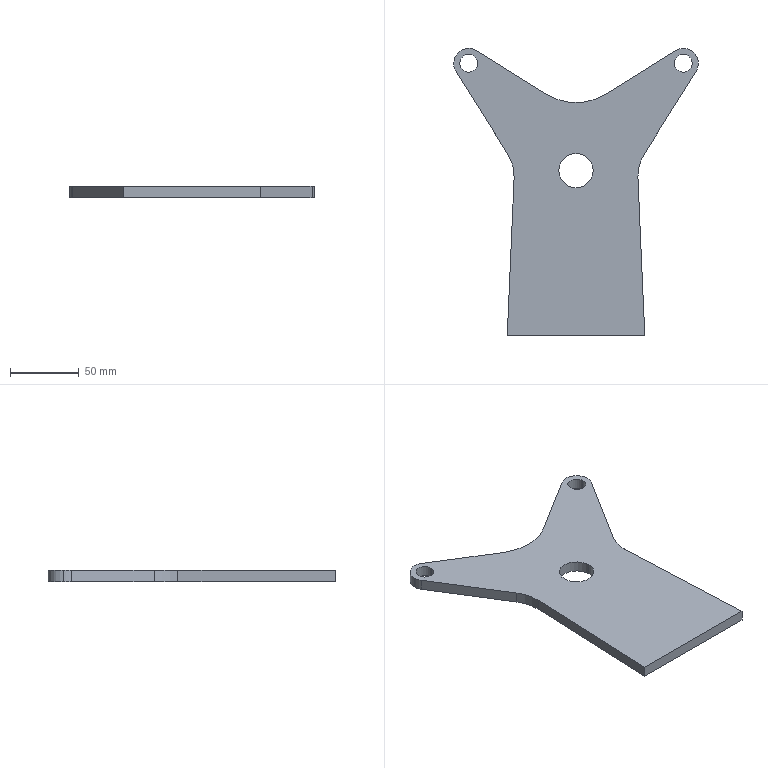Part | SolidWorks | features Extrusion 1 | 1 solid | 22 faces | box 177.818 x 208.909 x 8 mm | volume 156021 mm3 | cylinder 13 | plane 9 | commonest cylinder face diameters 13 x4 21.818 x3 60 x3 25 x2 80 x1
STEP:
#1=CARTESIAN_POINT('',(-84.5,198.,4.));
#2=VERTEX_POINT('',#1);
#3=CARTESIAN_POINT('',(-71.5,198.,4.));
#4=VERTEX_POINT('',#3);
#5=CARTESIAN_POINT('',(-78.,198.,4.));
#6=DIRECTION('',(0.,0.,1.));
#7=DIRECTION('',(-1.,0.,0.));
#8=AXIS2_PLACEMENT_3D('',#5,#6,#7);
#9=CIRCLE('',#8,6.5);
#10=EDGE_CURVE('',#2,#4,#9,.T.);
#11=ORIENTED_EDGE('',*,*,#10,.T.);
#12=CARTESIAN_POINT('',(-71.5,198.,-4.));
#13=VERTEX_POINT('',#12);
#14=CARTESIAN_POINT('',(-71.5,198.,4.));
#15=DIRECTION('',(0.,0.,-1.));
#16=VECTOR('',#15,1000.);
#17=LINE('',#14,#16);
#18=EDGE_CURVE('',#4,#13,#17,.T.);
#19=ORIENTED_EDGE('',*,*,#18,.T.);
#20=CARTESIAN_POINT('',(-84.5,198.,-4.));
#21=VERTEX_POINT('',#20);
#22=CARTESIAN_POINT('',(-78.,198.,-4.));
#23=DIRECTION('',(0.,0.,1.));
#24=DIRECTION('',(-1.,0.,0.));
#25=AXIS2_PLACEMENT_3D('',#22,#23,#24);
#26=CIRCLE('',#25,6.5);
#27=EDGE_CURVE('',#21,#13,#26,.T.);
#28=ORIENTED_EDGE('',*,*,#27,.F.);
#29=CARTESIAN_POINT('',(-84.5,198.,4.));
#30=DIRECTION('',(0.,0.,-1.));
#31=VECTOR('',#30,1000.);
#32=LINE('',#29,#31);
#33=EDGE_CURVE('',#2,#21,#32,.T.);
#34=ORIENTED_EDGE('',*,*,#33,.F.);
#35=EDGE_LOOP('',(#11,#19,#28,#34));
#36=FACE_OUTER_BOUND('',#35,.T.);
#37=CARTESIAN_POINT('',(-78.,198.,4.));
#38=DIRECTION('',(0.,0.,-1.));
#39=DIRECTION('',(-1.,0.,0.));
#40=AXIS2_PLACEMENT_3D('',#37,#38,#39);
#41=CYLINDRICAL_SURFACE('',#40,6.5);
#42=ADVANCED_FACE('',(#36),#41,.F.);
#43=CARTESIAN_POINT('',(-12.5,120.,4.));
#44=VERTEX_POINT('',#43);
#45=CARTESIAN_POINT('',(12.5,120.,4.));
#46=VERTEX_POINT('',#45);
#47=CARTESIAN_POINT('',(0.,120.,4.));
#48=DIRECTION('',(0.,0.,1.));
#49=DIRECTION('',(1.,0.,0.));
#50=AXIS2_PLACEMENT_3D('',#47,#48,#49);
#51=CIRCLE('',#50,12.5);
#52=EDGE_CURVE('',#44,#46,#51,.T.);
#53=ORIENTED_EDGE('',*,*,#52,.T.);
#54=CARTESIAN_POINT('',(12.5,120.,-4.));
#55=VERTEX_POINT('',#54);
#56=CARTESIAN_POINT('',(12.5,120.,4.));
#57=DIRECTION('',(0.,0.,-1.));
#58=VECTOR('',#57,1000.);
#59=LINE('',#56,#58);
#60=EDGE_CURVE('',#46,#55,#59,.T.);
#61=ORIENTED_EDGE('',*,*,#60,.T.);
#62=CARTESIAN_POINT('',(-12.5,120.,-4.));
#63=VERTEX_POINT('',#62);
#64=CARTESIAN_POINT('',(0.,120.,-4.));
#65=DIRECTION('',(0.,0.,1.));
#66=DIRECTION('',(1.,0.,0.));
#67=AXIS2_PLACEMENT_3D('',#64,#65,#66);
#68=CIRCLE('',#67,12.5);
#69=EDGE_CURVE('',#63,#55,#68,.T.);
#70=ORIENTED_EDGE('',*,*,#69,.F.);
#71=CARTESIAN_POINT('',(-12.5,120.,4.));
#72=DIRECTION('',(0.,0.,-1.));
#73=VECTOR('',#72,1000.);
#74=LINE('',#71,#73);
#75=EDGE_CURVE('',#44,#63,#74,.T.);
#76=ORIENTED_EDGE('',*,*,#75,.F.);
#77=EDGE_LOOP('',(#53,#61,#70,#76));
#78=FACE_OUTER_BOUND('',#77,.T.);
#79=CARTESIAN_POINT('',(0.,120.,4.));
#80=DIRECTION('',(0.,0.,-1.));
#81=DIRECTION('',(-1.,0.,0.));
#82=AXIS2_PLACEMENT_3D('',#79,#80,#81);
#83=CYLINDRICAL_SURFACE('',#82,12.5);
#84=ADVANCED_FACE('',(#78),#83,.F.);
#85=CARTESIAN_POINT('',(71.5,198.,4.));
#86=VERTEX_POINT('',#85);
#87=CARTESIAN_POINT('',(84.5,198.,4.));
#88=VERTEX_POINT('',#87);
#89=CARTESIAN_POINT('',(78.,198.,4.));
#90=DIRECTION('',(0.,0.,1.));
#91=DIRECTION('',(1.,0.,0.));
#92=AXIS2_PLACEMENT_3D('',#89,#90,#91);
#93=CIRCLE('',#92,6.5);
#94=EDGE_CURVE('',#86,#88,#93,.T.);
#95=ORIENTED_EDGE('',*,*,#94,.T.);
#96=CARTESIAN_POINT('',(84.5,198.,-4.));
#97=VERTEX_POINT('',#96);
#98=CARTESIAN_POINT('',(84.5,198.,4.));
#99=DIRECTION('',(0.,0.,-1.));
#100=VECTOR('',#99,1000.);
#101=LINE('',#98,#100);
#102=EDGE_CURVE('',#88,#97,#101,.T.);
#103=ORIENTED_EDGE('',*,*,#102,.T.);
#104=CARTESIAN_POINT('',(71.5,198.,-4.));
#105=VERTEX_POINT('',#104);
#106=CARTESIAN_POINT('',(78.,198.,-4.));
#107=DIRECTION('',(0.,0.,1.));
#108=DIRECTION('',(1.,0.,0.));
#109=AXIS2_PLACEMENT_3D('',#106,#107,#108);
#110=CIRCLE('',#109,6.5);
#111=EDGE_CURVE('',#105,#97,#110,.T.);
#112=ORIENTED_EDGE('',*,*,#111,.F.);
#113=CARTESIAN_POINT('',(71.5,198.,4.));
#114=DIRECTION('',(0.,0.,-1.));
#115=VECTOR('',#114,1000.);
#116=LINE('',#113,#115);
#117=EDGE_CURVE('',#86,#105,#116,.T.);
#118=ORIENTED_EDGE('',*,*,#117,.F.);
#119=EDGE_LOOP('',(#95,#103,#112,#118));
#120=FACE_OUTER_BOUND('',#119,.T.);
#121=CARTESIAN_POINT('',(78.,198.,4.));
#122=DIRECTION('',(0.,0.,-1.));
#123=DIRECTION('',(-1.,0.,0.));
#124=AXIS2_PLACEMENT_3D('',#121,#122,#123);
#125=CYLINDRICAL_SURFACE('',#124,6.5);
#126=ADVANCED_FACE('',(#120),#125,.F.);
#127=CARTESIAN_POINT('',(-88.909,198.,4.));
#128=VERTEX_POINT('',#127);
#129=CARTESIAN_POINT('',(-87.252,192.219,4.));
#130=VERTEX_POINT('',#129);
#131=CARTESIAN_POINT('',(-78.,198.,4.));
#132=DIRECTION('',(0.,0.,1.));
#133=DIRECTION('',(-1.,0.,0.));
#134=AXIS2_PLACEMENT_3D('',#131,#132,#133);
#135=CIRCLE('',#134,10.909);
#136=EDGE_CURVE('',#128,#130,#135,.T.);
#137=ORIENTED_EDGE('',*,*,#136,.F.);
#138=CARTESIAN_POINT('',(-88.909,198.,-4.));
#139=VERTEX_POINT('',#138);
#140=CARTESIAN_POINT('',(-88.909,198.,4.));
#141=DIRECTION('',(0.,0.,-1.));
#142=VECTOR('',#141,1000.);
#143=LINE('',#140,#142);
#144=EDGE_CURVE('',#128,#139,#143,.T.);
#145=ORIENTED_EDGE('',*,*,#144,.T.);
#146=CARTESIAN_POINT('',(-87.252,192.219,-4.));
#147=VERTEX_POINT('',#146);
#148=CARTESIAN_POINT('',(-78.,198.,-4.));
#149=DIRECTION('',(0.,0.,1.));
#150=DIRECTION('',(-1.,0.,0.));
#151=AXIS2_PLACEMENT_3D('',#148,#149,#150);
#152=CIRCLE('',#151,10.909);
#153=EDGE_CURVE('',#139,#147,#152,.T.);
#154=ORIENTED_EDGE('',*,*,#153,.T.);
#155=CARTESIAN_POINT('',(-87.252,192.219,4.));
#156=DIRECTION('',(0.,0.,-1.));
#157=VECTOR('',#156,1000.);
#158=LINE('',#155,#157);
#159=EDGE_CURVE('',#130,#147,#158,.T.);
#160=ORIENTED_EDGE('',*,*,#159,.F.);
#161=EDGE_LOOP('',(#137,#145,#154,#160));
#162=FACE_OUTER_BOUND('',#161,.T.);
#163=CARTESIAN_POINT('',(-78.,198.,4.));
#164=DIRECTION('',(0.,0.,-1.));
#165=DIRECTION('',(-1.,0.,0.));
#166=AXIS2_PLACEMENT_3D('',#163,#164,#165);
#167=CYLINDRICAL_SURFACE('',#166,10.909);
#168=ADVANCED_FACE('',(#162),#167,.T.);
#169=CARTESIAN_POINT('',(45.,116.,4.));
#170=VERTEX_POINT('',#169);
#171=CARTESIAN_POINT('',(49.559,131.898,4.));
#172=VERTEX_POINT('',#171);
#173=CARTESIAN_POINT('',(75.,116.,4.));
#174=DIRECTION('',(0.,0.,-1.));
#175=DIRECTION('',(-1.,0.,0.));
#176=AXIS2_PLACEMENT_3D('',#173,#174,#175);
#177=CIRCLE('',#176,30.);
#178=EDGE_CURVE('',#170,#172,#177,.T.);
#179=ORIENTED_EDGE('',*,*,#178,.F.);
#180=CARTESIAN_POINT('',(45.,116.,-4.));
#181=VERTEX_POINT('',#180);
#182=CARTESIAN_POINT('',(45.,116.,4.));
#183=DIRECTION('',(0.,0.,-1.));
#184=VECTOR('',#183,1000.);
#185=LINE('',#182,#184);
#186=EDGE_CURVE('',#170,#181,#185,.T.);
#187=ORIENTED_EDGE('',*,*,#186,.T.);
#188=CARTESIAN_POINT('',(49.559,131.898,-4.));
#189=VERTEX_POINT('',#188);
#190=CARTESIAN_POINT('',(75.,116.,-4.));
#191=DIRECTION('',(0.,0.,-1.));
#192=DIRECTION('',(-1.,0.,0.));
#193=AXIS2_PLACEMENT_3D('',#190,#191,#192);
#194=CIRCLE('',#193,30.);
#195=EDGE_CURVE('',#181,#189,#194,.T.);
#196=ORIENTED_EDGE('',*,*,#195,.T.);
#197=CARTESIAN_POINT('',(49.559,131.898,4.));
#198=DIRECTION('',(0.,0.,-1.));
#199=VECTOR('',#198,1000.);
#200=LINE('',#197,#199);
#201=EDGE_CURVE('',#172,#189,#200,.T.);
#202=ORIENTED_EDGE('',*,*,#201,.F.);
#203=EDGE_LOOP('',(#179,#187,#196,#202));
#204=FACE_OUTER_BOUND('',#203,.T.);
#205=CARTESIAN_POINT('',(75.,116.,4.));
#206=DIRECTION('',(0.,0.,-1.));
#207=DIRECTION('',(-1.,0.,0.));
#208=AXIS2_PLACEMENT_3D('',#205,#206,#207);
#209=CYLINDRICAL_SURFACE('',#208,30.);
#210=ADVANCED_FACE('',(#204),#209,.F.);
#211=ORIENTED_EDGE('',*,*,#52,.F.);
#212=CARTESIAN_POINT('',(0.,120.,4.));
#213=DIRECTION('',(0.,0.,1.));
#214=DIRECTION('',(1.,0.,0.));
#215=AXIS2_PLACEMENT_3D('',#212,#213,#214);
#216=CIRCLE('',#215,12.5);
#217=EDGE_CURVE('',#46,#44,#216,.T.);
#218=ORIENTED_EDGE('',*,*,#217,.F.);
#219=EDGE_LOOP('',(#211,#218));
#220=FACE_BOUND('',#219,.T.);
#221=CARTESIAN_POINT('',(-45.028,114.701,4.));
#222=VERTEX_POINT('',#221);
#223=CARTESIAN_POINT('',(-50.,0.,4.));
#224=VERTEX_POINT('',#223);
#225=CARTESIAN_POINT('',(-50.,0.,4.));
#226=DIRECTION('',(-0.04331,-0.9991,0.));
#227=VECTOR('',#226,1000.);
#228=LINE('',#225,#227);
#229=EDGE_CURVE('',#222,#224,#228,.T.);
#230=ORIENTED_EDGE('',*,*,#229,.T.);
#231=CARTESIAN_POINT('',(50.,0.,4.));
#232=VERTEX_POINT('',#231);
#233=CARTESIAN_POINT('',(50.,0.,4.));
#234=DIRECTION('',(1.,0.,0.));
#235=VECTOR('',#234,1000.);
#236=LINE('',#233,#235);
#237=EDGE_CURVE('',#224,#232,#236,.T.);
#238=ORIENTED_EDGE('',*,*,#237,.T.);
#239=CARTESIAN_POINT('',(45.028,114.701,4.));
#240=VERTEX_POINT('',#239);
#241=CARTESIAN_POINT('',(50.,0.,4.));
#242=DIRECTION('',(-0.04331,0.9991,0.));
#243=VECTOR('',#242,1000.);
#244=LINE('',#241,#243);
#245=EDGE_CURVE('',#232,#240,#244,.T.);
#246=ORIENTED_EDGE('',*,*,#245,.T.);
#247=CARTESIAN_POINT('',(75.,116.,4.));
#248=DIRECTION('',(0.,0.,-1.));
#249=DIRECTION('',(-1.,0.,0.));
#250=AXIS2_PLACEMENT_3D('',#247,#248,#249);
#251=CIRCLE('',#250,30.);
#252=EDGE_CURVE('',#240,#170,#251,.T.);
#253=ORIENTED_EDGE('',*,*,#252,.T.);
#254=ORIENTED_EDGE('',*,*,#178,.T.);
#255=CARTESIAN_POINT('',(87.252,192.219,4.));
#256=VERTEX_POINT('',#255);
#257=CARTESIAN_POINT('',(49.559,131.898,4.));
#258=DIRECTION('',(0.5299,0.848,0.));
#259=VECTOR('',#258,1000.);
#260=LINE('',#257,#259);
#261=EDGE_CURVE('',#172,#256,#260,.T.);
#262=ORIENTED_EDGE('',*,*,#261,.T.);
#263=CARTESIAN_POINT('',(72.219,207.252,4.));
#264=VERTEX_POINT('',#263);
#265=CARTESIAN_POINT('',(78.,198.,4.));
#266=DIRECTION('',(0.,0.,1.));
#267=DIRECTION('',(1.,0.,0.));
#268=AXIS2_PLACEMENT_3D('',#265,#266,#267);
#269=CIRCLE('',#268,10.909);
#270=EDGE_CURVE('',#256,#264,#269,.T.);
#271=ORIENTED_EDGE('',*,*,#270,.T.);
#272=CARTESIAN_POINT('',(21.197,175.369,4.));
#273=VERTEX_POINT('',#272);
#274=CARTESIAN_POINT('',(72.219,207.252,4.));
#275=DIRECTION('',(-0.848,-0.5299,0.));
#276=VECTOR('',#275,1000.);
#277=LINE('',#274,#276);
#278=EDGE_CURVE('',#264,#273,#277,.T.);
#279=ORIENTED_EDGE('',*,*,#278,.T.);
#280=CARTESIAN_POINT('',(-21.197,175.369,4.));
#281=VERTEX_POINT('',#280);
#282=CARTESIAN_POINT('',(0.,209.291,4.));
#283=DIRECTION('',(0.,0.,-1.));
#284=DIRECTION('',(-1.,0.,0.));
#285=AXIS2_PLACEMENT_3D('',#282,#283,#284);
#286=CIRCLE('',#285,40.);
#287=EDGE_CURVE('',#273,#281,#286,.T.);
#288=ORIENTED_EDGE('',*,*,#287,.T.);
#289=CARTESIAN_POINT('',(-72.219,207.252,4.));
#290=VERTEX_POINT('',#289);
#291=CARTESIAN_POINT('',(-72.219,207.252,4.));
#292=DIRECTION('',(-0.848,0.5299,0.));
#293=VECTOR('',#292,1000.);
#294=LINE('',#291,#293);
#295=EDGE_CURVE('',#281,#290,#294,.T.);
#296=ORIENTED_EDGE('',*,*,#295,.T.);
#297=CARTESIAN_POINT('',(-78.,198.,4.));
#298=DIRECTION('',(0.,0.,1.));
#299=DIRECTION('',(-1.,0.,0.));
#300=AXIS2_PLACEMENT_3D('',#297,#298,#299);
#301=CIRCLE('',#300,10.909);
#302=EDGE_CURVE('',#290,#128,#301,.T.);
#303=ORIENTED_EDGE('',*,*,#302,.T.);
#304=ORIENTED_EDGE('',*,*,#136,.T.);
#305=CARTESIAN_POINT('',(-49.559,131.898,4.));
#306=VERTEX_POINT('',#305);
#307=CARTESIAN_POINT('',(-49.559,131.898,4.));
#308=DIRECTION('',(0.5299,-0.848,0.));
#309=VECTOR('',#308,1000.);
#310=LINE('',#307,#309);
#311=EDGE_CURVE('',#130,#306,#310,.T.);
#312=ORIENTED_EDGE('',*,*,#311,.T.);
#313=CARTESIAN_POINT('',(-75.,116.,4.));
#314=DIRECTION('',(0.,0.,-1.));
#315=DIRECTION('',(1.,0.,0.));
#316=AXIS2_PLACEMENT_3D('',#313,#314,#315);
#317=CIRCLE('',#316,30.);
#318=EDGE_CURVE('',#306,#222,#317,.T.);
#319=ORIENTED_EDGE('',*,*,#318,.T.);
#320=EDGE_LOOP('',(#230,#238,#246,#253,#254,#262,#271,#279,#288,#296,#303,#304,#312,#319));
#321=FACE_OUTER_BOUND('',#320,.T.);
#322=ORIENTED_EDGE('',*,*,#94,.F.);
#323=CARTESIAN_POINT('',(78.,198.,4.));
#324=DIRECTION('',(0.,0.,1.));
#325=DIRECTION('',(1.,0.,0.));
#326=AXIS2_PLACEMENT_3D('',#323,#324,#325);
#327=CIRCLE('',#326,6.5);
#328=EDGE_CURVE('',#88,#86,#327,.T.);
#329=ORIENTED_EDGE('',*,*,#328,.F.);
#330=EDGE_LOOP('',(#322,#329));
#331=FACE_BOUND('',#330,.T.);
#332=ORIENTED_EDGE('',*,*,#10,.F.);
#333=CARTESIAN_POINT('',(-78.,198.,4.));
#334=DIRECTION('',(0.,0.,1.));
#335=DIRECTION('',(-1.,0.,0.));
#336=AXIS2_PLACEMENT_3D('',#333,#334,#335);
#337=CIRCLE('',#336,6.5);
#338=EDGE_CURVE('',#4,#2,#337,.T.);
#339=ORIENTED_EDGE('',*,*,#338,.F.);
#340=EDGE_LOOP('',(#332,#339));
#341=FACE_BOUND('',#340,.T.);
#342=CARTESIAN_POINT('',(-75.,116.,4.));
#343=DIRECTION('',(0.,0.,1.));
#344=DIRECTION('',(1.,0.,0.));
#345=AXIS2_PLACEMENT_3D('',#342,#343,#344);
#346=PLANE('',#345);
#347=ADVANCED_FACE('',(#220,#321,#331,#341),#346,.T.);
#348=CARTESIAN_POINT('',(-45.028,114.701,-4.));
#349=VERTEX_POINT('',#348);
#350=CARTESIAN_POINT('',(-50.,0.,-4.));
#351=VERTEX_POINT('',#350);
#352=CARTESIAN_POINT('',(-50.,0.,-4.));
#353=DIRECTION('',(-0.04331,-0.9991,0.));
#354=VECTOR('',#353,1000.);
#355=LINE('',#352,#354);
#356=EDGE_CURVE('',#349,#351,#355,.T.);
#357=ORIENTED_EDGE('',*,*,#356,.F.);
#358=CARTESIAN_POINT('',(-49.559,131.898,-4.));
#359=VERTEX_POINT('',#358);
#360=CARTESIAN_POINT('',(-75.,116.,-4.));
#361=DIRECTION('',(0.,0.,-1.));
#362=DIRECTION('',(1.,0.,0.));
#363=AXIS2_PLACEMENT_3D('',#360,#361,#362);
#364=CIRCLE('',#363,30.);
#365=EDGE_CURVE('',#359,#349,#364,.T.);
#366=ORIENTED_EDGE('',*,*,#365,.F.);
#367=CARTESIAN_POINT('',(-49.559,131.898,-4.));
#368=DIRECTION('',(0.5299,-0.848,0.));
#369=VECTOR('',#368,1000.);
#370=LINE('',#367,#369);
#371=EDGE_CURVE('',#147,#359,#370,.T.);
#372=ORIENTED_EDGE('',*,*,#371,.F.);
#373=ORIENTED_EDGE('',*,*,#153,.F.);
#374=CARTESIAN_POINT('',(-72.219,207.252,-4.));
#375=VERTEX_POINT('',#374);
#376=CARTESIAN_POINT('',(-78.,198.,-4.));
#377=DIRECTION('',(0.,0.,1.));
#378=DIRECTION('',(-1.,0.,0.));
#379=AXIS2_PLACEMENT_3D('',#376,#377,#378);
#380=CIRCLE('',#379,10.909);
#381=EDGE_CURVE('',#375,#139,#380,.T.);
#382=ORIENTED_EDGE('',*,*,#381,.F.);
#383=CARTESIAN_POINT('',(-21.197,175.369,-4.));
#384=VERTEX_POINT('',#383);
#385=CARTESIAN_POINT('',(-72.219,207.252,-4.));
#386=DIRECTION('',(-0.848,0.5299,0.));
#387=VECTOR('',#386,1000.);
#388=LINE('',#385,#387);
#389=EDGE_CURVE('',#384,#375,#388,.T.);
#390=ORIENTED_EDGE('',*,*,#389,.F.);
#391=CARTESIAN_POINT('',(21.197,175.369,-4.));
#392=VERTEX_POINT('',#391);
#393=CARTESIAN_POINT('',(0.,209.291,-4.));
#394=DIRECTION('',(0.,0.,-1.));
#395=DIRECTION('',(1.,0.,0.));
#396=AXIS2_PLACEMENT_3D('',#393,#394,#395);
#397=CIRCLE('',#396,40.);
#398=EDGE_CURVE('',#392,#384,#397,.T.);
#399=ORIENTED_EDGE('',*,*,#398,.F.);
#400=CARTESIAN_POINT('',(72.219,207.252,-4.));
#401=VERTEX_POINT('',#400);
#402=CARTESIAN_POINT('',(72.219,207.252,-4.));
#403=DIRECTION('',(-0.848,-0.5299,0.));
#404=VECTOR('',#403,1000.);
#405=LINE('',#402,#404);
#406=EDGE_CURVE('',#401,#392,#405,.T.);
#407=ORIENTED_EDGE('',*,*,#406,.F.);
#408=CARTESIAN_POINT('',(87.252,192.219,-4.));
#409=VERTEX_POINT('',#408);
#410=CARTESIAN_POINT('',(78.,198.,-4.));
#411=DIRECTION('',(0.,0.,1.));
#412=DIRECTION('',(1.,0.,0.));
#413=AXIS2_PLACEMENT_3D('',#410,#411,#412);
#414=CIRCLE('',#413,10.909);
#415=EDGE_CURVE('',#409,#401,#414,.T.);
#416=ORIENTED_EDGE('',*,*,#415,.F.);
#417=CARTESIAN_POINT('',(49.559,131.898,-4.));
#418=DIRECTION('',(0.5299,0.848,0.));
#419=VECTOR('',#418,1000.);
#420=LINE('',#417,#419);
#421=EDGE_CURVE('',#189,#409,#420,.T.);
#422=ORIENTED_EDGE('',*,*,#421,.F.);
#423=ORIENTED_EDGE('',*,*,#195,.F.);
#424=CARTESIAN_POINT('',(45.028,114.701,-4.));
#425=VERTEX_POINT('',#424);
#426=CARTESIAN_POINT('',(75.,116.,-4.));
#427=DIRECTION('',(0.,0.,-1.));
#428=DIRECTION('',(-1.,0.,0.));
#429=AXIS2_PLACEMENT_3D('',#426,#427,#428);
#430=CIRCLE('',#429,30.);
#431=EDGE_CURVE('',#425,#181,#430,.T.);
#432=ORIENTED_EDGE('',*,*,#431,.F.);
#433=CARTESIAN_POINT('',(50.,0.,-4.));
#434=VERTEX_POINT('',#433);
#435=CARTESIAN_POINT('',(50.,0.,-4.));
#436=DIRECTION('',(-0.04331,0.9991,0.));
#437=VECTOR('',#436,1000.);
#438=LINE('',#435,#437);
#439=EDGE_CURVE('',#434,#425,#438,.T.);
#440=ORIENTED_EDGE('',*,*,#439,.F.);
#441=CARTESIAN_POINT('',(50.,0.,-4.));
#442=DIRECTION('',(1.,0.,0.));
#443=VECTOR('',#442,1000.);
#444=LINE('',#441,#443);
#445=EDGE_CURVE('',#351,#434,#444,.T.);
#446=ORIENTED_EDGE('',*,*,#445,.F.);
#447=EDGE_LOOP('',(#357,#366,#372,#373,#382,#390,#399,#407,#416,#422,#423,#432,#440,#446));
#448=FACE_OUTER_BOUND('',#447,.T.);
#449=ORIENTED_EDGE('',*,*,#111,.T.);
#450=CARTESIAN_POINT('',(78.,198.,-4.));
#451=DIRECTION('',(0.,0.,1.));
#452=DIRECTION('',(1.,0.,0.));
#453=AXIS2_PLACEMENT_3D('',#450,#451,#452);
#454=CIRCLE('',#453,6.5);
#455=EDGE_CURVE('',#97,#105,#454,.T.);
#456=ORIENTED_EDGE('',*,*,#455,.T.);
#457=EDGE_LOOP('',(#449,#456));
#458=FACE_BOUND('',#457,.T.);
#459=ORIENTED_EDGE('',*,*,#69,.T.);
#460=CARTESIAN_POINT('',(0.,120.,-4.));
#461=DIRECTION('',(0.,0.,1.));
#462=DIRECTION('',(1.,0.,0.));
#463=AXIS2_PLACEMENT_3D('',#460,#461,#462);
#464=CIRCLE('',#463,12.5);
#465=EDGE_CURVE('',#55,#63,#464,.T.);
#466=ORIENTED_EDGE('',*,*,#465,.T.);
#467=EDGE_LOOP('',(#459,#466));
#468=FACE_BOUND('',#467,.T.);
#469=ORIENTED_EDGE('',*,*,#27,.T.);
#470=CARTESIAN_POINT('',(-78.,198.,-4.));
#471=DIRECTION('',(0.,0.,1.));
#472=DIRECTION('',(-1.,0.,0.));
#473=AXIS2_PLACEMENT_3D('',#470,#471,#472);
#474=CIRCLE('',#473,6.5);
#475=EDGE_CURVE('',#13,#21,#474,.T.);
#476=ORIENTED_EDGE('',*,*,#475,.T.);
#477=EDGE_LOOP('',(#469,#476));
#478=FACE_BOUND('',#477,.T.);
#479=CARTESIAN_POINT('',(-75.,116.,-4.));
#480=DIRECTION('',(0.,0.,1.));
#481=DIRECTION('',(1.,0.,0.));
#482=AXIS2_PLACEMENT_3D('',#479,#480,#481);
#483=PLANE('',#482);
#484=ADVANCED_FACE('',(#448,#458,#468,#478),#483,.F.);
#485=ORIENTED_EDGE('',*,*,#356,.T.);
#486=CARTESIAN_POINT('',(-50.,0.,4.));
#487=DIRECTION('',(0.,0.,-1.));
#488=VECTOR('',#487,1000.);
#489=LINE('',#486,#488);
#490=EDGE_CURVE('',#224,#351,#489,.T.);
#491=ORIENTED_EDGE('',*,*,#490,.F.);
#492=ORIENTED_EDGE('',*,*,#229,.F.);
#493=CARTESIAN_POINT('',(-45.028,114.701,4.));
#494=DIRECTION('',(0.,0.,-1.));
#495=VECTOR('',#494,1000.);
#496=LINE('',#493,#495);
#497=EDGE_CURVE('',#222,#349,#496,.T.);
#498=ORIENTED_EDGE('',*,*,#497,.T.);
#499=EDGE_LOOP('',(#485,#491,#492,#498));
#500=FACE_OUTER_BOUND('',#499,.T.);
#501=CARTESIAN_POINT('',(-50.,0.,4.));
#502=DIRECTION('',(0.9991,-0.04331,0.));
#503=DIRECTION('',(0.04331,0.9991,0.));
#504=AXIS2_PLACEMENT_3D('',#501,#502,#503);
#505=PLANE('',#504);
#506=ADVANCED_FACE('',(#500),#505,.F.);
#507=ORIENTED_EDGE('',*,*,#445,.T.);
#508=CARTESIAN_POINT('',(50.,0.,4.));
#509=DIRECTION('',(0.,0.,-1.));
#510=VECTOR('',#509,1000.);
#511=LINE('',#508,#510);
#512=EDGE_CURVE('',#232,#434,#511,.T.);
#513=ORIENTED_EDGE('',*,*,#512,.F.);
#514=ORIENTED_EDGE('',*,*,#237,.F.);
#515=ORIENTED_EDGE('',*,*,#490,.T.);
#516=EDGE_LOOP('',(#507,#513,#514,#515));
#517=FACE_OUTER_BOUND('',#516,.T.);
#518=CARTESIAN_POINT('',(50.,0.,4.));
#519=DIRECTION('',(0.,1.,0.));
#520=DIRECTION('',(0.,0.,1.));
#521=AXIS2_PLACEMENT_3D('',#518,#519,#520);
#522=PLANE('',#521);
#523=ADVANCED_FACE('',(#517),#522,.F.);
#524=ORIENTED_EDGE('',*,*,#439,.T.);
#525=CARTESIAN_POINT('',(45.028,114.701,4.));
#526=DIRECTION('',(0.,0.,-1.));
#527=VECTOR('',#526,1000.);
#528=LINE('',#525,#527);
#529=EDGE_CURVE('',#240,#425,#528,.T.);
#530=ORIENTED_EDGE('',*,*,#529,.F.);
#531=ORIENTED_EDGE('',*,*,#245,.F.);
#532=ORIENTED_EDGE('',*,*,#512,.T.);
#533=EDGE_LOOP('',(#524,#530,#531,#532));
#534=FACE_OUTER_BOUND('',#533,.T.);
#535=CARTESIAN_POINT('',(50.,0.,4.));
#536=DIRECTION('',(-0.9991,-0.04331,0.));
#537=DIRECTION('',(0.04331,-0.9991,0.));
#538=AXIS2_PLACEMENT_3D('',#535,#536,#537);
#539=PLANE('',#538);
#540=ADVANCED_FACE('',(#534),#539,.F.);
#541=ORIENTED_EDGE('',*,*,#186,.F.);
#542=ORIENTED_EDGE('',*,*,#252,.F.);
#543=ORIENTED_EDGE('',*,*,#529,.T.);
#544=ORIENTED_EDGE('',*,*,#431,.T.);
#545=EDGE_LOOP('',(#541,#542,#543,#544));
#546=FACE_OUTER_BOUND('',#545,.T.);
#547=CARTESIAN_POINT('',(75.,116.,4.));
#548=DIRECTION('',(0.,0.,-1.));
#549=DIRECTION('',(-1.,0.,0.));
#550=AXIS2_PLACEMENT_3D('',#547,#548,#549);
#551=CYLINDRICAL_SURFACE('',#550,30.);
#552=ADVANCED_FACE('',(#546),#551,.F.);
#553=ORIENTED_EDGE('',*,*,#421,.T.);
#554=CARTESIAN_POINT('',(87.252,192.219,4.));
#555=DIRECTION('',(0.,0.,-1.));
#556=VECTOR('',#555,1000.);
#557=LINE('',#554,#556);
#558=EDGE_CURVE('',#256,#409,#557,.T.);
#559=ORIENTED_EDGE('',*,*,#558,.F.);
#560=ORIENTED_EDGE('',*,*,#261,.F.);
#561=ORIENTED_EDGE('',*,*,#201,.T.);
#562=EDGE_LOOP('',(#553,#559,#560,#561));
#563=FACE_OUTER_BOUND('',#562,.T.);
#564=CARTESIAN_POINT('',(49.559,131.898,4.));
#565=DIRECTION('',(-0.848,0.5299,0.));
#566=DIRECTION('',(-0.5299,-0.848,0.));
#567=AXIS2_PLACEMENT_3D('',#564,#565,#566);
#568=PLANE('',#567);
#569=ADVANCED_FACE('',(#563),#568,.F.);
#570=ORIENTED_EDGE('',*,*,#415,.T.);
#571=CARTESIAN_POINT('',(72.219,207.252,4.));
#572=DIRECTION('',(0.,0.,-1.));
#573=VECTOR('',#572,1000.);
#574=LINE('',#571,#573);
#575=EDGE_CURVE('',#264,#401,#574,.T.);
#576=ORIENTED_EDGE('',*,*,#575,.F.);
#577=ORIENTED_EDGE('',*,*,#270,.F.);
#578=ORIENTED_EDGE('',*,*,#558,.T.);
#579=EDGE_LOOP('',(#570,#576,#577,#578));
#580=FACE_OUTER_BOUND('',#579,.T.);
#581=CARTESIAN_POINT('',(78.,198.,4.));
#582=DIRECTION('',(0.,0.,-1.));
#583=DIRECTION('',(-1.,0.,0.));
#584=AXIS2_PLACEMENT_3D('',#581,#582,#583);
#585=CYLINDRICAL_SURFACE('',#584,10.909);
#586=ADVANCED_FACE('',(#580),#585,.T.);
#587=ORIENTED_EDGE('',*,*,#406,.T.);
#588=CARTESIAN_POINT('',(21.197,175.369,4.));
#589=DIRECTION('',(0.,0.,-1.));
#590=VECTOR('',#589,1000.);
#591=LINE('',#588,#590);
#592=EDGE_CURVE('',#273,#392,#591,.T.);
#593=ORIENTED_EDGE('',*,*,#592,.F.);
#594=ORIENTED_EDGE('',*,*,#278,.F.);
#595=ORIENTED_EDGE('',*,*,#575,.T.);
#596=EDGE_LOOP('',(#587,#593,#594,#595));
#597=FACE_OUTER_BOUND('',#596,.T.);
#598=CARTESIAN_POINT('',(72.219,207.252,4.));
#599=DIRECTION('',(0.5299,-0.848,0.));
#600=DIRECTION('',(0.848,0.5299,0.));
#601=AXIS2_PLACEMENT_3D('',#598,#599,#600);
#602=PLANE('',#601);
#603=ADVANCED_FACE('',(#597),#602,.F.);
#604=ORIENTED_EDGE('',*,*,#398,.T.);
#605=CARTESIAN_POINT('',(-21.197,175.369,4.));
#606=DIRECTION('',(0.,0.,-1.));
#607=VECTOR('',#606,1000.);
#608=LINE('',#605,#607);
#609=EDGE_CURVE('',#281,#384,#608,.T.);
#610=ORIENTED_EDGE('',*,*,#609,.F.);
#611=ORIENTED_EDGE('',*,*,#287,.F.);
#612=ORIENTED_EDGE('',*,*,#592,.T.);
#613=EDGE_LOOP('',(#604,#610,#611,#612));
#614=FACE_OUTER_BOUND('',#613,.T.);
#615=CARTESIAN_POINT('',(0.,209.291,4.));
#616=DIRECTION('',(0.,0.,-1.));
#617=DIRECTION('',(-1.,0.,0.));
#618=AXIS2_PLACEMENT_3D('',#615,#616,#617);
#619=CYLINDRICAL_SURFACE('',#618,40.);
#620=ADVANCED_FACE('',(#614),#619,.F.);
#621=ORIENTED_EDGE('',*,*,#389,.T.);
#622=CARTESIAN_POINT('',(-72.219,207.252,4.));
#623=DIRECTION('',(0.,0.,-1.));
#624=VECTOR('',#623,1000.);
#625=LINE('',#622,#624);
#626=EDGE_CURVE('',#290,#375,#625,.T.);
#627=ORIENTED_EDGE('',*,*,#626,.F.);
#628=ORIENTED_EDGE('',*,*,#295,.F.);
#629=ORIENTED_EDGE('',*,*,#609,.T.);
#630=EDGE_LOOP('',(#621,#627,#628,#629));
#631=FACE_OUTER_BOUND('',#630,.T.);
#632=CARTESIAN_POINT('',(-72.219,207.252,4.));
#633=DIRECTION('',(-0.5299,-0.848,0.));
#634=DIRECTION('',(0.848,-0.5299,0.));
#635=AXIS2_PLACEMENT_3D('',#632,#633,#634);
#636=PLANE('',#635);
#637=ADVANCED_FACE('',(#631),#636,.F.);
#638=ORIENTED_EDGE('',*,*,#144,.F.);
#639=ORIENTED_EDGE('',*,*,#302,.F.);
#640=ORIENTED_EDGE('',*,*,#626,.T.);
#641=ORIENTED_EDGE('',*,*,#381,.T.);
#642=EDGE_LOOP('',(#638,#639,#640,#641));
#643=FACE_OUTER_BOUND('',#642,.T.);
#644=CARTESIAN_POINT('',(-78.,198.,4.));
#645=DIRECTION('',(0.,0.,-1.));
#646=DIRECTION('',(-1.,0.,0.));
#647=AXIS2_PLACEMENT_3D('',#644,#645,#646);
#648=CYLINDRICAL_SURFACE('',#647,10.909);
#649=ADVANCED_FACE('',(#643),#648,.T.);
#650=ORIENTED_EDGE('',*,*,#371,.T.);
#651=CARTESIAN_POINT('',(-49.559,131.898,4.));
#652=DIRECTION('',(0.,0.,-1.));
#653=VECTOR('',#652,1000.);
#654=LINE('',#651,#653);
#655=EDGE_CURVE('',#306,#359,#654,.T.);
#656=ORIENTED_EDGE('',*,*,#655,.F.);
#657=ORIENTED_EDGE('',*,*,#311,.F.);
#658=ORIENTED_EDGE('',*,*,#159,.T.);
#659=EDGE_LOOP('',(#650,#656,#657,#658));
#660=FACE_OUTER_BOUND('',#659,.T.);
#661=CARTESIAN_POINT('',(-49.559,131.898,4.));
#662=DIRECTION('',(0.848,0.5299,0.));
#663=DIRECTION('',(-0.5299,0.848,0.));
#664=AXIS2_PLACEMENT_3D('',#661,#662,#663);
#665=PLANE('',#664);
#666=ADVANCED_FACE('',(#660),#665,.F.);
#667=ORIENTED_EDGE('',*,*,#365,.T.);
#668=ORIENTED_EDGE('',*,*,#497,.F.);
#669=ORIENTED_EDGE('',*,*,#318,.F.);
#670=ORIENTED_EDGE('',*,*,#655,.T.);
#671=EDGE_LOOP('',(#667,#668,#669,#670));
#672=FACE_OUTER_BOUND('',#671,.T.);
#673=CARTESIAN_POINT('',(-75.,116.,4.));
#674=DIRECTION('',(0.,0.,-1.));
#675=DIRECTION('',(-1.,0.,0.));
#676=AXIS2_PLACEMENT_3D('',#673,#674,#675);
#677=CYLINDRICAL_SURFACE('',#676,30.);
#678=ADVANCED_FACE('',(#672),#677,.F.);
#679=ORIENTED_EDGE('',*,*,#102,.F.);
#680=ORIENTED_EDGE('',*,*,#328,.T.);
#681=ORIENTED_EDGE('',*,*,#117,.T.);
#682=ORIENTED_EDGE('',*,*,#455,.F.);
#683=EDGE_LOOP('',(#679,#680,#681,#682));
#684=FACE_OUTER_BOUND('',#683,.T.);
#685=CARTESIAN_POINT('',(78.,198.,4.));
#686=DIRECTION('',(0.,0.,-1.));
#687=DIRECTION('',(-1.,0.,0.));
#688=AXIS2_PLACEMENT_3D('',#685,#686,#687);
#689=CYLINDRICAL_SURFACE('',#688,6.5);
#690=ADVANCED_FACE('',(#684),#689,.F.);
#691=ORIENTED_EDGE('',*,*,#60,.F.);
#692=ORIENTED_EDGE('',*,*,#217,.T.);
#693=ORIENTED_EDGE('',*,*,#75,.T.);
#694=ORIENTED_EDGE('',*,*,#465,.F.);
#695=EDGE_LOOP('',(#691,#692,#693,#694));
#696=FACE_OUTER_BOUND('',#695,.T.);
#697=CARTESIAN_POINT('',(0.,120.,4.));
#698=DIRECTION('',(0.,0.,-1.));
#699=DIRECTION('',(-1.,0.,0.));
#700=AXIS2_PLACEMENT_3D('',#697,#698,#699);
#701=CYLINDRICAL_SURFACE('',#700,12.5);
#702=ADVANCED_FACE('',(#696),#701,.F.);
#703=ORIENTED_EDGE('',*,*,#18,.F.);
#704=ORIENTED_EDGE('',*,*,#338,.T.);
#705=ORIENTED_EDGE('',*,*,#33,.T.);
#706=ORIENTED_EDGE('',*,*,#475,.F.);
#707=EDGE_LOOP('',(#703,#704,#705,#706));
#708=FACE_OUTER_BOUND('',#707,.T.);
#709=CARTESIAN_POINT('',(-78.,198.,4.));
#710=DIRECTION('',(0.,0.,-1.));
#711=DIRECTION('',(-1.,0.,0.));
#712=AXIS2_PLACEMENT_3D('',#709,#710,#711);
#713=CYLINDRICAL_SURFACE('',#712,6.5);
#714=ADVANCED_FACE('',(#708),#713,.F.);
#715=CLOSED_SHELL('',(#42,#84,#126,#168,#210,#347,#484,#506,#523,#540,#552,#569,#586,#603,#620,#637,#649,#666,#678,#690,#702,#714));
#716=MANIFOLD_SOLID_BREP('',#715);
#717=CARTESIAN_POINT('',(0.,0.,0.));
#718=DIRECTION('',(0.,0.,1.));
#719=DIRECTION('',(1.,0.,0.));
#720=AXIS2_PLACEMENT_3D('',#717,#718,#719);
#721=(LENGTH_UNIT()NAMED_UNIT(*)SI_UNIT(.MILLI.,.METRE.));
#722=UNCERTAINTY_MEASURE_WITH_UNIT(LENGTH_MEASURE(0.00001),#721,'','');
#723=(NAMED_UNIT(*)PLANE_ANGLE_UNIT()SI_UNIT($,.RADIAN.));
#724=(NAMED_UNIT(*)SI_UNIT($,.STERADIAN.)SOLID_ANGLE_UNIT());
#725=(GEOMETRIC_REPRESENTATION_CONTEXT(3)GLOBAL_UNCERTAINTY_ASSIGNED_CONTEXT((#722))GLOBAL_UNIT_ASSIGNED_CONTEXT((#721,#723,#724))REPRESENTATION_CONTEXT('',''));
#726=ADVANCED_BREP_SHAPE_REPRESENTATION('',(#716,#720),#725);